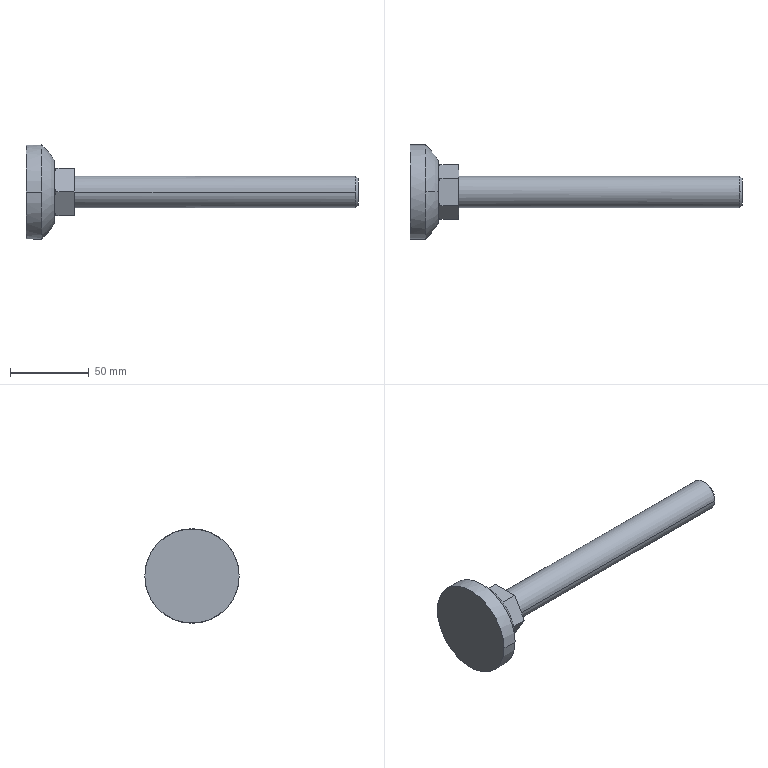Part | STEP file | 1 solid | 38 faces | box 211 x 60 x 60 mm | volume 110948 mm3 | plane 22 | cone 10 | cylinder 4 | other 2 | commonest cylinder face diameters 20 x2 60 x2